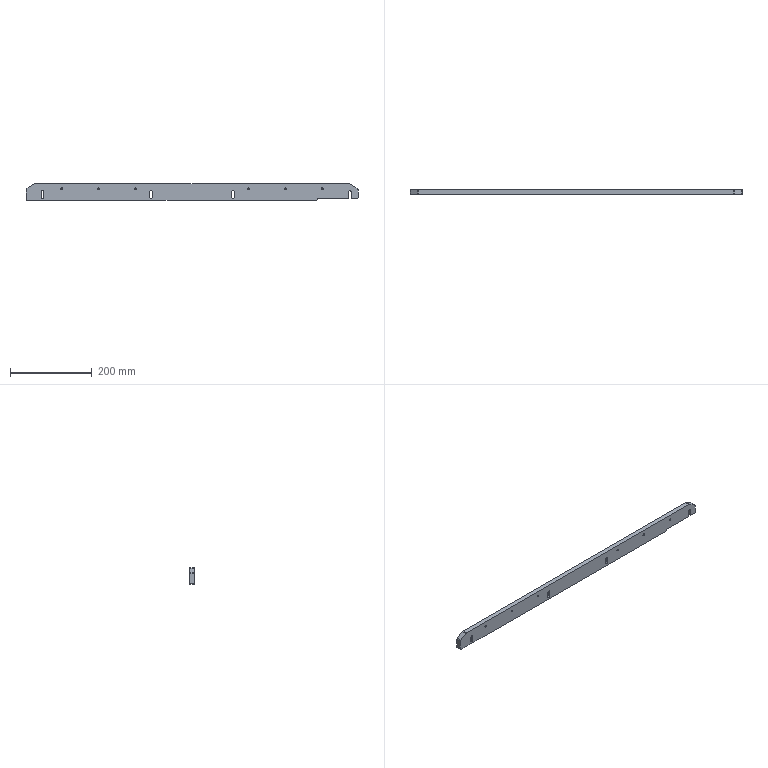Part | 1 solid | 58 faces | box 810 x 12 x 40 mm | volume 369950 mm3 | plane 34 | cylinder 24 | commonest cylinder face diameters 6.6 x7 11 x7 5 x6 10 x4